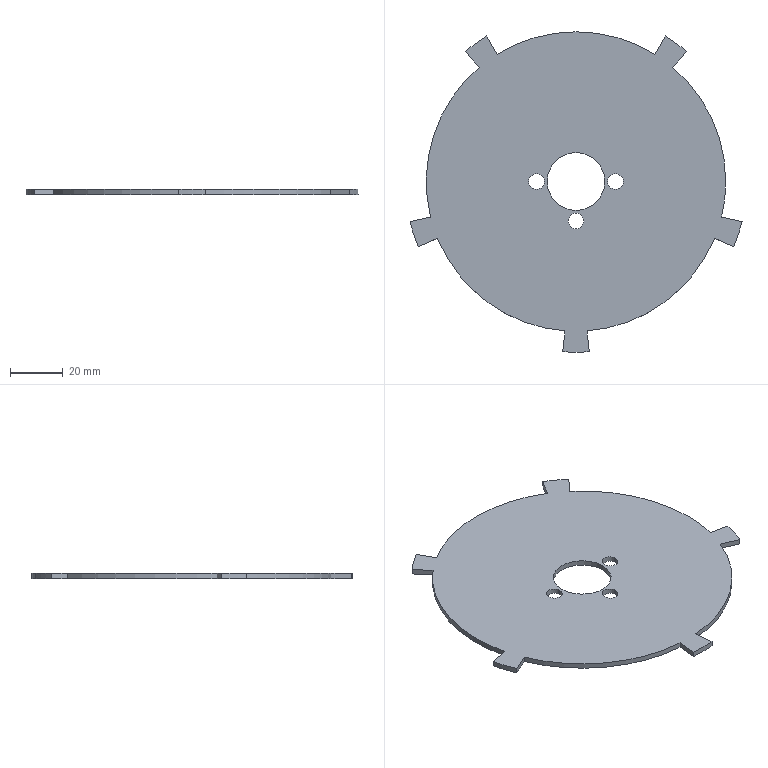Part | STEP file | 1004-2001-0084_1004-2001-0084_1-2 | 1 solid | 31 faces | box 126.387 x 122 x 2 mm | volume 20227 mm3 | cylinder 19 | plane 12 | commonest cylinder face diameters 6 x6 114 x6 130 x5 22 x2
STEP:
#1=CARTESIAN_POINT('',(-11.,0.,-1.));
#2=VERTEX_POINT('',#1);
#3=CARTESIAN_POINT('',(11.,0.,-1.));
#4=VERTEX_POINT('',#3);
#5=CARTESIAN_POINT('',(0.,0.,-1.));
#6=DIRECTION('',(0.,0.,1.));
#7=DIRECTION('',(1.,0.,0.));
#8=AXIS2_PLACEMENT_3D('',#5,#6,#7);
#9=CIRCLE('',#8,11.);
#10=EDGE_CURVE('',#2,#4,#9,.T.);
#11=ORIENTED_EDGE('',*,*,#10,.F.);
#12=CARTESIAN_POINT('',(-11.,0.,1.));
#13=VERTEX_POINT('',#12);
#14=CARTESIAN_POINT('',(-11.,0.,1.));
#15=DIRECTION('',(0.,0.,1.));
#16=VECTOR('',#15,1000.);
#17=LINE('',#14,#16);
#18=EDGE_CURVE('',#2,#13,#17,.T.);
#19=ORIENTED_EDGE('',*,*,#18,.T.);
#20=CARTESIAN_POINT('',(11.,0.,1.));
#21=VERTEX_POINT('',#20);
#22=CARTESIAN_POINT('',(0.,0.,1.));
#23=DIRECTION('',(0.,0.,-1.));
#24=DIRECTION('',(1.,0.,0.));
#25=AXIS2_PLACEMENT_3D('',#22,#23,#24);
#26=CIRCLE('',#25,11.);
#27=EDGE_CURVE('',#21,#13,#26,.T.);
#28=ORIENTED_EDGE('',*,*,#27,.F.);
#29=CARTESIAN_POINT('',(11.,0.,1.));
#30=DIRECTION('',(0.,0.,1.));
#31=VECTOR('',#30,1000.);
#32=LINE('',#29,#31);
#33=EDGE_CURVE('',#4,#21,#32,.T.);
#34=ORIENTED_EDGE('',*,*,#33,.F.);
#35=EDGE_LOOP('',(#11,#19,#28,#34));
#36=FACE_OUTER_BOUND('',#35,.T.);
#37=CARTESIAN_POINT('',(0.,0.,1.));
#38=DIRECTION('',(0.,0.,1.));
#39=DIRECTION('',(1.,0.,0.));
#40=AXIS2_PLACEMENT_3D('',#37,#38,#39);
#41=CYLINDRICAL_SURFACE('',#40,11.);
#42=ADVANCED_FACE('',(#36),#41,.F.);
#43=CARTESIAN_POINT('',(3.,-15.,1.));
#44=VERTEX_POINT('',#43);
#45=CARTESIAN_POINT('',(-3.,-15.,1.));
#46=VERTEX_POINT('',#45);
#47=CARTESIAN_POINT('',(0.,-15.,1.));
#48=DIRECTION('',(0.,0.,-1.));
#49=DIRECTION('',(-1.,0.,0.));
#50=AXIS2_PLACEMENT_3D('',#47,#48,#49);
#51=CIRCLE('',#50,3.);
#52=EDGE_CURVE('',#44,#46,#51,.T.);
#53=ORIENTED_EDGE('',*,*,#52,.F.);
#54=CARTESIAN_POINT('',(3.,-15.,-1.));
#55=VERTEX_POINT('',#54);
#56=CARTESIAN_POINT('',(3.,-15.,-1.));
#57=DIRECTION('',(0.,0.,-1.));
#58=VECTOR('',#57,1000.);
#59=LINE('',#56,#58);
#60=EDGE_CURVE('',#44,#55,#59,.T.);
#61=ORIENTED_EDGE('',*,*,#60,.T.);
#62=CARTESIAN_POINT('',(-3.,-15.,-1.));
#63=VERTEX_POINT('',#62);
#64=CARTESIAN_POINT('',(0.,-15.,-1.));
#65=DIRECTION('',(0.,0.,1.));
#66=DIRECTION('',(-1.,0.,0.));
#67=AXIS2_PLACEMENT_3D('',#64,#65,#66);
#68=CIRCLE('',#67,3.);
#69=EDGE_CURVE('',#63,#55,#68,.T.);
#70=ORIENTED_EDGE('',*,*,#69,.F.);
#71=CARTESIAN_POINT('',(-3.,-15.,-1.));
#72=DIRECTION('',(0.,0.,-1.));
#73=VECTOR('',#72,1000.);
#74=LINE('',#71,#73);
#75=EDGE_CURVE('',#46,#63,#74,.T.);
#76=ORIENTED_EDGE('',*,*,#75,.F.);
#77=EDGE_LOOP('',(#53,#61,#70,#76));
#78=FACE_OUTER_BOUND('',#77,.T.);
#79=CARTESIAN_POINT('',(0.,-15.,-1.));
#80=DIRECTION('',(0.,0.,-1.));
#81=DIRECTION('',(-1.,0.,0.));
#82=AXIS2_PLACEMENT_3D('',#79,#80,#81);
#83=CYLINDRICAL_SURFACE('',#82,3.);
#84=ADVANCED_FACE('',(#78),#83,.F.);
#85=CARTESIAN_POINT('',(-12.,0.,1.));
#86=VERTEX_POINT('',#85);
#87=CARTESIAN_POINT('',(-18.,0.,1.));
#88=VERTEX_POINT('',#87);
#89=CARTESIAN_POINT('',(-15.,0.,1.));
#90=DIRECTION('',(0.,0.,-1.));
#91=DIRECTION('',(-1.,0.,0.));
#92=AXIS2_PLACEMENT_3D('',#89,#90,#91);
#93=CIRCLE('',#92,3.);
#94=EDGE_CURVE('',#86,#88,#93,.T.);
#95=ORIENTED_EDGE('',*,*,#94,.F.);
#96=CARTESIAN_POINT('',(-12.,0.,-1.));
#97=VERTEX_POINT('',#96);
#98=CARTESIAN_POINT('',(-12.,0.,-1.));
#99=DIRECTION('',(0.,0.,-1.));
#100=VECTOR('',#99,1000.);
#101=LINE('',#98,#100);
#102=EDGE_CURVE('',#86,#97,#101,.T.);
#103=ORIENTED_EDGE('',*,*,#102,.T.);
#104=CARTESIAN_POINT('',(-18.,0.,-1.));
#105=VERTEX_POINT('',#104);
#106=CARTESIAN_POINT('',(-15.,0.,-1.));
#107=DIRECTION('',(0.,0.,1.));
#108=DIRECTION('',(-1.,0.,0.));
#109=AXIS2_PLACEMENT_3D('',#106,#107,#108);
#110=CIRCLE('',#109,3.);
#111=EDGE_CURVE('',#105,#97,#110,.T.);
#112=ORIENTED_EDGE('',*,*,#111,.F.);
#113=CARTESIAN_POINT('',(-18.,0.,-1.));
#114=DIRECTION('',(0.,0.,-1.));
#115=VECTOR('',#114,1000.);
#116=LINE('',#113,#115);
#117=EDGE_CURVE('',#88,#105,#116,.T.);
#118=ORIENTED_EDGE('',*,*,#117,.F.);
#119=EDGE_LOOP('',(#95,#103,#112,#118));
#120=FACE_OUTER_BOUND('',#119,.T.);
#121=CARTESIAN_POINT('',(-15.,0.,-1.));
#122=DIRECTION('',(0.,0.,-1.));
#123=DIRECTION('',(-1.,0.,0.));
#124=AXIS2_PLACEMENT_3D('',#121,#122,#123);
#125=CYLINDRICAL_SURFACE('',#124,3.);
#126=ADVANCED_FACE('',(#120),#125,.F.);
#127=CARTESIAN_POINT('',(18.,0.,1.));
#128=VERTEX_POINT('',#127);
#129=CARTESIAN_POINT('',(12.,0.,1.));
#130=VERTEX_POINT('',#129);
#131=CARTESIAN_POINT('',(15.,0.,1.));
#132=DIRECTION('',(0.,0.,-1.));
#133=DIRECTION('',(-1.,0.,0.));
#134=AXIS2_PLACEMENT_3D('',#131,#132,#133);
#135=CIRCLE('',#134,3.);
#136=EDGE_CURVE('',#128,#130,#135,.T.);
#137=ORIENTED_EDGE('',*,*,#136,.F.);
#138=CARTESIAN_POINT('',(18.,0.,-1.));
#139=VERTEX_POINT('',#138);
#140=CARTESIAN_POINT('',(18.,0.,-1.));
#141=DIRECTION('',(0.,0.,-1.));
#142=VECTOR('',#141,1000.);
#143=LINE('',#140,#142);
#144=EDGE_CURVE('',#128,#139,#143,.T.);
#145=ORIENTED_EDGE('',*,*,#144,.T.);
#146=CARTESIAN_POINT('',(12.,0.,-1.));
#147=VERTEX_POINT('',#146);
#148=CARTESIAN_POINT('',(15.,0.,-1.));
#149=DIRECTION('',(0.,0.,1.));
#150=DIRECTION('',(-1.,0.,0.));
#151=AXIS2_PLACEMENT_3D('',#148,#149,#150);
#152=CIRCLE('',#151,3.);
#153=EDGE_CURVE('',#147,#139,#152,.T.);
#154=ORIENTED_EDGE('',*,*,#153,.F.);
#155=CARTESIAN_POINT('',(12.,0.,-1.));
#156=DIRECTION('',(0.,0.,-1.));
#157=VECTOR('',#156,1000.);
#158=LINE('',#155,#157);
#159=EDGE_CURVE('',#130,#147,#158,.T.);
#160=ORIENTED_EDGE('',*,*,#159,.F.);
#161=EDGE_LOOP('',(#137,#145,#154,#160));
#162=FACE_OUTER_BOUND('',#161,.T.);
#163=CARTESIAN_POINT('',(15.,0.,-1.));
#164=DIRECTION('',(0.,0.,-1.));
#165=DIRECTION('',(-1.,0.,0.));
#166=AXIS2_PLACEMENT_3D('',#163,#164,#165);
#167=CYLINDRICAL_SURFACE('',#166,3.);
#168=ADVANCED_FACE('',(#162),#167,.F.);
#169=CARTESIAN_POINT('',(55.365,-13.555,-1.));
#170=VERTEX_POINT('',#169);
#171=CARTESIAN_POINT('',(57.,0.,-1.));
#172=VERTEX_POINT('',#171);
#173=CARTESIAN_POINT('',(0.,0.,-1.));
#174=DIRECTION('',(0.,0.,1.));
#175=DIRECTION('',(1.,0.,0.));
#176=AXIS2_PLACEMENT_3D('',#173,#174,#175);
#177=CIRCLE('',#176,57.);
#178=EDGE_CURVE('',#170,#172,#177,.T.);
#179=ORIENTED_EDGE('',*,*,#178,.T.);
#180=CARTESIAN_POINT('',(57.,0.,1.));
#181=VERTEX_POINT('',#180);
#182=CARTESIAN_POINT('',(57.,0.,-1.));
#183=DIRECTION('',(0.,0.,1.));
#184=VECTOR('',#183,1000.);
#185=LINE('',#182,#184);
#186=EDGE_CURVE('',#172,#181,#185,.T.);
#187=ORIENTED_EDGE('',*,*,#186,.T.);
#188=CARTESIAN_POINT('',(55.365,-13.555,1.));
#189=VERTEX_POINT('',#188);
#190=CARTESIAN_POINT('',(0.,0.,1.));
#191=DIRECTION('',(0.,0.,1.));
#192=DIRECTION('',(1.,0.,0.));
#193=AXIS2_PLACEMENT_3D('',#190,#191,#192);
#194=CIRCLE('',#193,57.);
#195=EDGE_CURVE('',#189,#181,#194,.T.);
#196=ORIENTED_EDGE('',*,*,#195,.F.);
#197=CARTESIAN_POINT('',(55.365,-13.555,-1.));
#198=DIRECTION('',(0.,0.,-1.));
#199=VECTOR('',#198,1000.);
#200=LINE('',#197,#199);
#201=EDGE_CURVE('',#189,#170,#200,.T.);
#202=ORIENTED_EDGE('',*,*,#201,.T.);
#203=EDGE_LOOP('',(#179,#187,#196,#202));
#204=FACE_OUTER_BOUND('',#203,.T.);
#205=CARTESIAN_POINT('',(0.,0.,-1.));
#206=DIRECTION('',(0.,0.,1.));
#207=DIRECTION('',(1.,0.,0.));
#208=AXIS2_PLACEMENT_3D('',#205,#206,#207);
#209=CYLINDRICAL_SURFACE('',#208,57.);
#210=ADVANCED_FACE('',(#204),#209,.T.);
#211=ORIENTED_EDGE('',*,*,#27,.T.);
#212=CARTESIAN_POINT('',(0.,0.,1.));
#213=DIRECTION('',(0.,0.,-1.));
#214=DIRECTION('',(1.,0.,0.));
#215=AXIS2_PLACEMENT_3D('',#212,#213,#214);
#216=CIRCLE('',#215,11.);
#217=EDGE_CURVE('',#13,#21,#216,.T.);
#218=ORIENTED_EDGE('',*,*,#217,.T.);
#219=EDGE_LOOP('',(#211,#218));
#220=FACE_BOUND('',#219,.T.);
#221=CARTESIAN_POINT('',(0.,-15.,1.));
#222=DIRECTION('',(0.,0.,-1.));
#223=DIRECTION('',(-1.,0.,0.));
#224=AXIS2_PLACEMENT_3D('',#221,#222,#223);
#225=CIRCLE('',#224,3.);
#226=EDGE_CURVE('',#46,#44,#225,.T.);
#227=ORIENTED_EDGE('',*,*,#226,.T.);
#228=ORIENTED_EDGE('',*,*,#52,.T.);
#229=EDGE_LOOP('',(#227,#228));
#230=FACE_BOUND('',#229,.T.);
#231=CARTESIAN_POINT('',(-15.,0.,1.));
#232=DIRECTION('',(0.,0.,-1.));
#233=DIRECTION('',(-1.,0.,0.));
#234=AXIS2_PLACEMENT_3D('',#231,#232,#233);
#235=CIRCLE('',#234,3.);
#236=EDGE_CURVE('',#88,#86,#235,.T.);
#237=ORIENTED_EDGE('',*,*,#236,.T.);
#238=ORIENTED_EDGE('',*,*,#94,.T.);
#239=EDGE_LOOP('',(#237,#238));
#240=FACE_BOUND('',#239,.T.);
#241=CARTESIAN_POINT('',(15.,0.,1.));
#242=DIRECTION('',(0.,0.,-1.));
#243=DIRECTION('',(-1.,0.,0.));
#244=AXIS2_PLACEMENT_3D('',#241,#242,#243);
#245=CIRCLE('',#244,3.);
#246=EDGE_CURVE('',#130,#128,#245,.T.);
#247=ORIENTED_EDGE('',*,*,#246,.T.);
#248=ORIENTED_EDGE('',*,*,#136,.T.);
#249=EDGE_LOOP('',(#247,#248));
#250=FACE_BOUND('',#249,.T.);
#251=CARTESIAN_POINT('',(-36.824,43.509,1.));
#252=VERTEX_POINT('',#251);
#253=CARTESIAN_POINT('',(-55.365,-13.555,1.));
#254=VERTEX_POINT('',#253);
#255=CARTESIAN_POINT('',(0.,0.,1.));
#256=DIRECTION('',(0.,0.,1.));
#257=DIRECTION('',(1.,0.,0.));
#258=AXIS2_PLACEMENT_3D('',#255,#256,#257);
#259=CIRCLE('',#258,57.);
#260=EDGE_CURVE('',#252,#254,#259,.T.);
#261=ORIENTED_EDGE('',*,*,#260,.T.);
#262=CARTESIAN_POINT('',(-63.193,-15.219,1.));
#263=VERTEX_POINT('',#262);
#264=CARTESIAN_POINT('',(-55.365,-13.555,1.));
#265=DIRECTION('',(-0.9781,-0.2079,0.));
#266=VECTOR('',#265,1000.);
#267=LINE('',#264,#266);
#268=EDGE_CURVE('',#254,#263,#267,.T.);
#269=ORIENTED_EDGE('',*,*,#268,.T.);
#270=CARTESIAN_POINT('',(-60.07,-24.832,1.));
#271=VERTEX_POINT('',#270);
#272=CARTESIAN_POINT('',(0.,0.,1.));
#273=DIRECTION('',(0.,0.,1.));
#274=DIRECTION('',(-1.,0.,0.));
#275=AXIS2_PLACEMENT_3D('',#272,#273,#274);
#276=CIRCLE('',#275,65.);
#277=EDGE_CURVE('',#263,#271,#276,.T.);
#278=ORIENTED_EDGE('',*,*,#277,.T.);
#279=CARTESIAN_POINT('',(-52.758,-21.577,1.));
#280=VERTEX_POINT('',#279);
#281=CARTESIAN_POINT('',(-60.07,-24.832,1.));
#282=DIRECTION('',(0.9135,0.4067,0.));
#283=VECTOR('',#282,1000.);
#284=LINE('',#281,#283);
#285=EDGE_CURVE('',#271,#280,#284,.T.);
#286=ORIENTED_EDGE('',*,*,#285,.T.);
#287=CARTESIAN_POINT('',(-4.217,-56.844,1.));
#288=VERTEX_POINT('',#287);
#289=CARTESIAN_POINT('',(0.,0.,1.));
#290=DIRECTION('',(0.,0.,1.));
#291=DIRECTION('',(1.,0.,0.));
#292=AXIS2_PLACEMENT_3D('',#289,#290,#291);
#293=CIRCLE('',#292,57.);
#294=EDGE_CURVE('',#280,#288,#293,.T.);
#295=ORIENTED_EDGE('',*,*,#294,.T.);
#296=CARTESIAN_POINT('',(-5.054,-64.803,1.));
#297=VERTEX_POINT('',#296);
#298=CARTESIAN_POINT('',(-4.217,-56.844,1.));
#299=DIRECTION('',(-0.1045,-0.9945,0.));
#300=VECTOR('',#299,1000.);
#301=LINE('',#298,#300);
#302=EDGE_CURVE('',#288,#297,#301,.T.);
#303=ORIENTED_EDGE('',*,*,#302,.T.);
#304=CARTESIAN_POINT('',(5.054,-64.803,1.));
#305=VERTEX_POINT('',#304);
#306=CARTESIAN_POINT('',(0.,0.,1.));
#307=DIRECTION('',(0.,0.,1.));
#308=DIRECTION('',(-1.,0.,0.));
#309=AXIS2_PLACEMENT_3D('',#306,#307,#308);
#310=CIRCLE('',#309,65.);
#311=EDGE_CURVE('',#297,#305,#310,.T.);
#312=ORIENTED_EDGE('',*,*,#311,.T.);
#313=CARTESIAN_POINT('',(4.217,-56.844,1.));
#314=VERTEX_POINT('',#313);
#315=CARTESIAN_POINT('',(5.054,-64.803,1.));
#316=DIRECTION('',(-0.1045,0.9945,0.));
#317=VECTOR('',#316,1000.);
#318=LINE('',#315,#317);
#319=EDGE_CURVE('',#305,#314,#318,.T.);
#320=ORIENTED_EDGE('',*,*,#319,.T.);
#321=CARTESIAN_POINT('',(52.758,-21.577,1.));
#322=VERTEX_POINT('',#321);
#323=CARTESIAN_POINT('',(0.,0.,1.));
#324=DIRECTION('',(0.,0.,1.));
#325=DIRECTION('',(1.,0.,0.));
#326=AXIS2_PLACEMENT_3D('',#323,#324,#325);
#327=CIRCLE('',#326,57.);
#328=EDGE_CURVE('',#314,#322,#327,.T.);
#329=ORIENTED_EDGE('',*,*,#328,.T.);
#330=CARTESIAN_POINT('',(60.07,-24.832,1.));
#331=VERTEX_POINT('',#330);
#332=CARTESIAN_POINT('',(52.758,-21.577,1.));
#333=DIRECTION('',(0.9135,-0.4067,0.));
#334=VECTOR('',#333,1000.);
#335=LINE('',#332,#334);
#336=EDGE_CURVE('',#322,#331,#335,.T.);
#337=ORIENTED_EDGE('',*,*,#336,.T.);
#338=CARTESIAN_POINT('',(63.193,-15.219,1.));
#339=VERTEX_POINT('',#338);
#340=CARTESIAN_POINT('',(0.,0.,1.));
#341=DIRECTION('',(0.,0.,1.));
#342=DIRECTION('',(-1.,0.,0.));
#343=AXIS2_PLACEMENT_3D('',#340,#341,#342);
#344=CIRCLE('',#343,65.);
#345=EDGE_CURVE('',#331,#339,#344,.T.);
#346=ORIENTED_EDGE('',*,*,#345,.T.);
#347=CARTESIAN_POINT('',(63.193,-15.219,1.));
#348=DIRECTION('',(-0.9781,0.2079,0.));
#349=VECTOR('',#348,1000.);
#350=LINE('',#347,#349);
#351=EDGE_CURVE('',#339,#189,#350,.T.);
#352=ORIENTED_EDGE('',*,*,#351,.T.);
#353=ORIENTED_EDGE('',*,*,#195,.T.);
#354=CARTESIAN_POINT('',(36.824,43.509,1.));
#355=VERTEX_POINT('',#354);
#356=CARTESIAN_POINT('',(0.,0.,1.));
#357=DIRECTION('',(0.,0.,1.));
#358=DIRECTION('',(1.,0.,0.));
#359=AXIS2_PLACEMENT_3D('',#356,#357,#358);
#360=CIRCLE('',#359,57.);
#361=EDGE_CURVE('',#181,#355,#360,.T.);
#362=ORIENTED_EDGE('',*,*,#361,.T.);
#363=CARTESIAN_POINT('',(42.179,49.456,1.));
#364=VERTEX_POINT('',#363);
#365=CARTESIAN_POINT('',(36.824,43.509,1.));
#366=DIRECTION('',(0.6691,0.7431,0.));
#367=VECTOR('',#366,1000.);
#368=LINE('',#365,#367);
#369=EDGE_CURVE('',#355,#364,#368,.T.);
#370=ORIENTED_EDGE('',*,*,#369,.T.);
#371=CARTESIAN_POINT('',(34.002,55.398,1.));
#372=VERTEX_POINT('',#371);
#373=CARTESIAN_POINT('',(0.,0.,1.));
#374=DIRECTION('',(0.,0.,1.));
#375=DIRECTION('',(-1.,0.,0.));
#376=AXIS2_PLACEMENT_3D('',#373,#374,#375);
#377=CIRCLE('',#376,65.);
#378=EDGE_CURVE('',#364,#372,#377,.T.);
#379=ORIENTED_EDGE('',*,*,#378,.T.);
#380=CARTESIAN_POINT('',(30.,48.466,1.));
#381=VERTEX_POINT('',#380);
#382=CARTESIAN_POINT('',(34.002,55.398,1.));
#383=DIRECTION('',(-0.5,-0.866,0.));
#384=VECTOR('',#383,1000.);
#385=LINE('',#382,#384);
#386=EDGE_CURVE('',#372,#381,#385,.T.);
#387=ORIENTED_EDGE('',*,*,#386,.T.);
#388=CARTESIAN_POINT('',(-30.,48.466,1.));
#389=VERTEX_POINT('',#388);
#390=CARTESIAN_POINT('',(0.,0.,1.));
#391=DIRECTION('',(0.,0.,1.));
#392=DIRECTION('',(1.,0.,0.));
#393=AXIS2_PLACEMENT_3D('',#390,#391,#392);
#394=CIRCLE('',#393,57.);
#395=EDGE_CURVE('',#381,#389,#394,.T.);
#396=ORIENTED_EDGE('',*,*,#395,.T.);
#397=CARTESIAN_POINT('',(-34.002,55.398,1.));
#398=VERTEX_POINT('',#397);
#399=CARTESIAN_POINT('',(-30.,48.466,1.));
#400=DIRECTION('',(-0.5,0.866,0.));
#401=VECTOR('',#400,1000.);
#402=LINE('',#399,#401);
#403=EDGE_CURVE('',#389,#398,#402,.T.);
#404=ORIENTED_EDGE('',*,*,#403,.T.);
#405=CARTESIAN_POINT('',(-42.179,49.456,1.));
#406=VERTEX_POINT('',#405);
#407=CARTESIAN_POINT('',(0.,0.,1.));
#408=DIRECTION('',(0.,0.,1.));
#409=DIRECTION('',(-1.,0.,0.));
#410=AXIS2_PLACEMENT_3D('',#407,#408,#409);
#411=CIRCLE('',#410,65.);
#412=EDGE_CURVE('',#398,#406,#411,.T.);
#413=ORIENTED_EDGE('',*,*,#412,.T.);
#414=CARTESIAN_POINT('',(-42.179,49.456,1.));
#415=DIRECTION('',(0.6691,-0.7431,0.));
#416=VECTOR('',#415,1000.);
#417=LINE('',#414,#416);
#418=EDGE_CURVE('',#406,#252,#417,.T.);
#419=ORIENTED_EDGE('',*,*,#418,.T.);
#420=EDGE_LOOP('',(#261,#269,#278,#286,#295,#303,#312,#320,#329,#337,#346,#352,#353,#362,#370,#379,#387,#396,#404,#413,#419));
#421=FACE_OUTER_BOUND('',#420,.T.);
#422=CARTESIAN_POINT('',(0.,0.,1.));
#423=DIRECTION('',(0.,0.,1.));
#424=DIRECTION('',(1.,0.,0.));
#425=AXIS2_PLACEMENT_3D('',#422,#423,#424);
#426=PLANE('',#425);
#427=ADVANCED_FACE('',(#220,#230,#240,#250,#421),#426,.T.);
#428=ORIENTED_EDGE('',*,*,#18,.F.);
#429=CARTESIAN_POINT('',(0.,0.,-1.));
#430=DIRECTION('',(0.,0.,1.));
#431=DIRECTION('',(1.,0.,0.));
#432=AXIS2_PLACEMENT_3D('',#429,#430,#431);
#433=CIRCLE('',#432,11.);
#434=EDGE_CURVE('',#4,#2,#433,.T.);
#435=ORIENTED_EDGE('',*,*,#434,.F.);
#436=ORIENTED_EDGE('',*,*,#33,.T.);
#437=ORIENTED_EDGE('',*,*,#217,.F.);
#438=EDGE_LOOP('',(#428,#435,#436,#437));
#439=FACE_OUTER_BOUND('',#438,.T.);
#440=CARTESIAN_POINT('',(0.,0.,1.));
#441=DIRECTION('',(0.,0.,1.));
#442=DIRECTION('',(1.,0.,0.));
#443=AXIS2_PLACEMENT_3D('',#440,#441,#442);
#444=CYLINDRICAL_SURFACE('',#443,11.);
#445=ADVANCED_FACE('',(#439),#444,.F.);
#446=ORIENTED_EDGE('',*,*,#60,.F.);
#447=ORIENTED_EDGE('',*,*,#226,.F.);
#448=ORIENTED_EDGE('',*,*,#75,.T.);
#449=CARTESIAN_POINT('',(0.,-15.,-1.));
#450=DIRECTION('',(0.,0.,1.));
#451=DIRECTION('',(-1.,0.,0.));
#452=AXIS2_PLACEMENT_3D('',#449,#450,#451);
#453=CIRCLE('',#452,3.);
#454=EDGE_CURVE('',#55,#63,#453,.T.);
#455=ORIENTED_EDGE('',*,*,#454,.F.);
#456=EDGE_LOOP('',(#446,#447,#448,#455));
#457=FACE_OUTER_BOUND('',#456,.T.);
#458=CARTESIAN_POINT('',(0.,-15.,-1.));
#459=DIRECTION('',(0.,0.,-1.));
#460=DIRECTION('',(-1.,0.,0.));
#461=AXIS2_PLACEMENT_3D('',#458,#459,#460);
#462=CYLINDRICAL_SURFACE('',#461,3.);
#463=ADVANCED_FACE('',(#457),#462,.F.);
#464=ORIENTED_EDGE('',*,*,#102,.F.);
#465=ORIENTED_EDGE('',*,*,#236,.F.);
#466=ORIENTED_EDGE('',*,*,#117,.T.);
#467=CARTESIAN_POINT('',(-15.,0.,-1.));
#468=DIRECTION('',(0.,0.,1.));
#469=DIRECTION('',(-1.,0.,0.));
#470=AXIS2_PLACEMENT_3D('',#467,#468,#469);
#471=CIRCLE('',#470,3.);
#472=EDGE_CURVE('',#97,#105,#471,.T.);
#473=ORIENTED_EDGE('',*,*,#472,.F.);
#474=EDGE_LOOP('',(#464,#465,#466,#473));
#475=FACE_OUTER_BOUND('',#474,.T.);
#476=CARTESIAN_POINT('',(-15.,0.,-1.));
#477=DIRECTION('',(0.,0.,-1.));
#478=DIRECTION('',(-1.,0.,0.));
#479=AXIS2_PLACEMENT_3D('',#476,#477,#478);
#480=CYLINDRICAL_SURFACE('',#479,3.);
#481=ADVANCED_FACE('',(#475),#480,.F.);
#482=ORIENTED_EDGE('',*,*,#144,.F.);
#483=ORIENTED_EDGE('',*,*,#246,.F.);
#484=ORIENTED_EDGE('',*,*,#159,.T.);
#485=CARTESIAN_POINT('',(15.,0.,-1.));
#486=DIRECTION('',(0.,0.,1.));
#487=DIRECTION('',(-1.,0.,0.));
#488=AXIS2_PLACEMENT_3D('',#485,#486,#487);
#489=CIRCLE('',#488,3.);
#490=EDGE_CURVE('',#139,#147,#489,.T.);
#491=ORIENTED_EDGE('',*,*,#490,.F.);
#492=EDGE_LOOP('',(#482,#483,#484,#491));
#493=FACE_OUTER_BOUND('',#492,.T.);
#494=CARTESIAN_POINT('',(15.,0.,-1.));
#495=DIRECTION('',(0.,0.,-1.));
#496=DIRECTION('',(-1.,0.,0.));
#497=AXIS2_PLACEMENT_3D('',#494,#495,#496);
#498=CYLINDRICAL_SURFACE('',#497,3.);
#499=ADVANCED_FACE('',(#493),#498,.F.);
#500=CARTESIAN_POINT('',(-63.193,-15.219,-1.));
#501=VERTEX_POINT('',#500);
#502=CARTESIAN_POINT('',(-55.365,-13.555,-1.));
#503=VERTEX_POINT('',#502);
#504=CARTESIAN_POINT('',(-55.365,-13.555,-1.));
#505=DIRECTION('',(0.9781,0.2079,0.));
#506=VECTOR('',#505,1000.);
#507=LINE('',#504,#506);
#508=EDGE_CURVE('',#501,#503,#507,.T.);
#509=ORIENTED_EDGE('',*,*,#508,.F.);
#510=CARTESIAN_POINT('',(-63.193,-15.219,-1.));
#511=DIRECTION('',(0.,0.,-1.));
#512=VECTOR('',#511,1000.);
#513=LINE('',#510,#512);
#514=EDGE_CURVE('',#263,#501,#513,.T.);
#515=ORIENTED_EDGE('',*,*,#514,.F.);
#516=ORIENTED_EDGE('',*,*,#268,.F.);
#517=CARTESIAN_POINT('',(-55.365,-13.555,-1.));
#518=DIRECTION('',(0.,0.,1.));
#519=VECTOR('',#518,1000.);
#520=LINE('',#517,#519);
#521=EDGE_CURVE('',#503,#254,#520,.T.);
#522=ORIENTED_EDGE('',*,*,#521,.F.);
#523=EDGE_LOOP('',(#509,#515,#516,#522));
#524=FACE_OUTER_BOUND('',#523,.T.);
#525=CARTESIAN_POINT('',(-55.365,-13.555,-1.));
#526=DIRECTION('',(0.2079,-0.9781,0.));
#527=DIRECTION('',(0.9781,0.2079,0.));
#528=AXIS2_PLACEMENT_3D('',#525,#526,#527);
#529=PLANE('',#528);
#530=ADVANCED_FACE('',(#524),#529,.F.);
#531=ORIENTED_EDGE('',*,*,#521,.T.);
#532=ORIENTED_EDGE('',*,*,#260,.F.);
#533=CARTESIAN_POINT('',(-36.824,43.509,-1.));
#534=VERTEX_POINT('',#533);
#535=CARTESIAN_POINT('',(-36.824,43.509,-1.));
#536=DIRECTION('',(0.,0.,-1.));
#537=VECTOR('',#536,1000.);
#538=LINE('',#535,#537);
#539=EDGE_CURVE('',#252,#534,#538,.T.);
#540=ORIENTED_EDGE('',*,*,#539,.T.);
#541=CARTESIAN_POINT('',(0.,0.,-1.));
#542=DIRECTION('',(0.,0.,1.));
#543=DIRECTION('',(1.,0.,0.));
#544=AXIS2_PLACEMENT_3D('',#541,#542,#543);
#545=CIRCLE('',#544,57.);
#546=EDGE_CURVE('',#534,#503,#545,.T.);
#547=ORIENTED_EDGE('',*,*,#546,.T.);
#548=EDGE_LOOP('',(#531,#532,#540,#547));
#549=FACE_OUTER_BOUND('',#548,.T.);
#550=CARTESIAN_POINT('',(0.,0.,-1.));
#551=DIRECTION('',(0.,0.,1.));
#552=DIRECTION('',(1.,0.,0.));
#553=AXIS2_PLACEMENT_3D('',#550,#551,#552);
#554=CYLINDRICAL_SURFACE('',#553,57.);
#555=ADVANCED_FACE('',(#549),#554,.T.);
#556=CARTESIAN_POINT('',(-42.179,49.456,-1.));
#557=VERTEX_POINT('',#556);
#558=CARTESIAN_POINT('',(-36.824,43.509,-1.));
#559=DIRECTION('',(-0.6691,0.7431,0.));
#560=VECTOR('',#559,1000.);
#561=LINE('',#558,#560);
#562=EDGE_CURVE('',#534,#557,#561,.T.);
#563=ORIENTED_EDGE('',*,*,#562,.F.);
#564=ORIENTED_EDGE('',*,*,#539,.F.);
#565=ORIENTED_EDGE('',*,*,#418,.F.);
#566=CARTESIAN_POINT('',(-42.179,49.456,-1.));
#567=DIRECTION('',(0.,0.,1.));
#568=VECTOR('',#567,1000.);
#569=LINE('',#566,#568);
#570=EDGE_CURVE('',#557,#406,#569,.T.);
#571=ORIENTED_EDGE('',*,*,#570,.F.);
#572=EDGE_LOOP('',(#563,#564,#565,#571));
#573=FACE_OUTER_BOUND('',#572,.T.);
#574=CARTESIAN_POINT('',(-36.824,43.509,-1.));
#575=DIRECTION('',(0.7431,0.6691,0.));
#576=DIRECTION('',(-0.6691,0.7431,0.));
#577=AXIS2_PLACEMENT_3D('',#574,#575,#576);
#578=PLANE('',#577);
#579=ADVANCED_FACE('',(#573),#578,.F.);
#580=CARTESIAN_POINT('',(-34.002,55.398,-1.));
#581=VERTEX_POINT('',#580);
#582=CARTESIAN_POINT('',(-34.002,55.398,1.));
#583=DIRECTION('',(0.,0.,-1.));
#584=VECTOR('',#583,1000.);
#585=LINE('',#582,#584);
#586=EDGE_CURVE('',#398,#581,#585,.T.);
#587=ORIENTED_EDGE('',*,*,#586,.T.);
#588=CARTESIAN_POINT('',(0.,0.,-1.));
#589=DIRECTION('',(0.,0.,1.));
#590=DIRECTION('',(-1.,0.,0.));
#591=AXIS2_PLACEMENT_3D('',#588,#589,#590);
#592=CIRCLE('',#591,65.);
#593=EDGE_CURVE('',#581,#557,#592,.T.);
#594=ORIENTED_EDGE('',*,*,#593,.T.);
#595=ORIENTED_EDGE('',*,*,#570,.T.);
#596=ORIENTED_EDGE('',*,*,#412,.F.);
#597=EDGE_LOOP('',(#587,#594,#595,#596));
#598=FACE_OUTER_BOUND('',#597,.T.);
#599=CARTESIAN_POINT('',(0.,0.,1.));
#600=DIRECTION('',(0.,0.,-1.));
#601=DIRECTION('',(-1.,0.,0.));
#602=AXIS2_PLACEMENT_3D('',#599,#600,#601);
#603=CYLINDRICAL_SURFACE('',#602,65.);
#604=ADVANCED_FACE('',(#598),#603,.T.);
#605=CARTESIAN_POINT('',(-30.,48.466,-1.));
#606=VERTEX_POINT('',#605);
#607=CARTESIAN_POINT('',(-30.,48.466,-1.));
#608=DIRECTION('',(0.5,-0.866,0.));
#609=VECTOR('',#608,1000.);
#610=LINE('',#607,#609);
#611=EDGE_CURVE('',#581,#606,#610,.T.);
#612=ORIENTED_EDGE('',*,*,#611,.F.);
#613=ORIENTED_EDGE('',*,*,#586,.F.);
#614=ORIENTED_EDGE('',*,*,#403,.F.);
#615=CARTESIAN_POINT('',(-30.,48.466,-1.));
#616=DIRECTION('',(0.,0.,1.));
#617=VECTOR('',#616,1000.);
#618=LINE('',#615,#617);
#619=EDGE_CURVE('',#606,#389,#618,.T.);
#620=ORIENTED_EDGE('',*,*,#619,.F.);
#621=EDGE_LOOP('',(#612,#613,#614,#620));
#622=FACE_OUTER_BOUND('',#621,.T.);
#623=CARTESIAN_POINT('',(-30.,48.466,-1.));
#624=DIRECTION('',(-0.866,-0.5,0.));
#625=DIRECTION('',(0.5,-0.866,0.));
#626=AXIS2_PLACEMENT_3D('',#623,#624,#625);
#627=PLANE('',#626);
#628=ADVANCED_FACE('',(#622),#627,.F.);
#629=ORIENTED_EDGE('',*,*,#619,.T.);
#630=ORIENTED_EDGE('',*,*,#395,.F.);
#631=CARTESIAN_POINT('',(30.,48.466,-1.));
#632=VERTEX_POINT('',#631);
#633=CARTESIAN_POINT('',(30.,48.466,-1.));
#634=DIRECTION('',(0.,0.,-1.));
#635=VECTOR('',#634,1000.);
#636=LINE('',#633,#635);
#637=EDGE_CURVE('',#381,#632,#636,.T.);
#638=ORIENTED_EDGE('',*,*,#637,.T.);
#639=CARTESIAN_POINT('',(0.,0.,-1.));
#640=DIRECTION('',(0.,0.,1.));
#641=DIRECTION('',(1.,0.,0.));
#642=AXIS2_PLACEMENT_3D('',#639,#640,#641);
#643=CIRCLE('',#642,57.);
#644=EDGE_CURVE('',#632,#606,#643,.T.);
#645=ORIENTED_EDGE('',*,*,#644,.T.);
#646=EDGE_LOOP('',(#629,#630,#638,#645));
#647=FACE_OUTER_BOUND('',#646,.T.);
#648=CARTESIAN_POINT('',(0.,0.,-1.));
#649=DIRECTION('',(0.,0.,1.));
#650=DIRECTION('',(1.,0.,0.));
#651=AXIS2_PLACEMENT_3D('',#648,#649,#650);
#652=CYLINDRICAL_SURFACE('',#651,57.);
#653=ADVANCED_FACE('',(#647),#652,.T.);
#654=CARTESIAN_POINT('',(34.002,55.398,-1.));
#655=VERTEX_POINT('',#654);
#656=CARTESIAN_POINT('',(30.,48.466,-1.));
#657=DIRECTION('',(0.5,0.866,0.));
#658=VECTOR('',#657,1000.);
#659=LINE('',#656,#658);
#660=EDGE_CURVE('',#632,#655,#659,.T.);
#661=ORIENTED_EDGE('',*,*,#660,.F.);
#662=ORIENTED_EDGE('',*,*,#637,.F.);
#663=ORIENTED_EDGE('',*,*,#386,.F.);
#664=CARTESIAN_POINT('',(34.002,55.398,-1.));
#665=DIRECTION('',(0.,0.,1.));
#666=VECTOR('',#665,1000.);
#667=LINE('',#664,#666);
#668=EDGE_CURVE('',#655,#372,#667,.T.);
#669=ORIENTED_EDGE('',*,*,#668,.F.);
#670=EDGE_LOOP('',(#661,#662,#663,#669));
#671=FACE_OUTER_BOUND('',#670,.T.);
#672=CARTESIAN_POINT('',(30.,48.466,-1.));
#673=DIRECTION('',(0.866,-0.5,0.));
#674=DIRECTION('',(0.5,0.866,0.));
#675=AXIS2_PLACEMENT_3D('',#672,#673,#674);
#676=PLANE('',#675);
#677=ADVANCED_FACE('',(#671),#676,.F.);
#678=ORIENTED_EDGE('',*,*,#668,.T.);
#679=ORIENTED_EDGE('',*,*,#378,.F.);
#680=CARTESIAN_POINT('',(42.179,49.456,-1.));
#681=VERTEX_POINT('',#680);
#682=CARTESIAN_POINT('',(42.179,49.456,1.));
#683=DIRECTION('',(0.,0.,-1.));
#684=VECTOR('',#683,1000.);
#685=LINE('',#682,#684);
#686=EDGE_CURVE('',#364,#681,#685,.T.);
#687=ORIENTED_EDGE('',*,*,#686,.T.);
#688=CARTESIAN_POINT('',(0.,0.,-1.));
#689=DIRECTION('',(0.,0.,1.));
#690=DIRECTION('',(-1.,0.,0.));
#691=AXIS2_PLACEMENT_3D('',#688,#689,#690);
#692=CIRCLE('',#691,65.);
#693=EDGE_CURVE('',#681,#655,#692,.T.);
#694=ORIENTED_EDGE('',*,*,#693,.T.);
#695=EDGE_LOOP('',(#678,#679,#687,#694));
#696=FACE_OUTER_BOUND('',#695,.T.);
#697=CARTESIAN_POINT('',(0.,0.,1.));
#698=DIRECTION('',(0.,0.,-1.));
#699=DIRECTION('',(-1.,0.,0.));
#700=AXIS2_PLACEMENT_3D('',#697,#698,#699);
#701=CYLINDRICAL_SURFACE('',#700,65.);
#702=ADVANCED_FACE('',(#696),#701,.T.);
#703=CARTESIAN_POINT('',(36.824,43.509,-1.));
#704=VERTEX_POINT('',#703);
#705=CARTESIAN_POINT('',(36.824,43.509,-1.));
#706=DIRECTION('',(-0.6691,-0.7431,0.));
#707=VECTOR('',#706,1000.);
#708=LINE('',#705,#707);
#709=EDGE_CURVE('',#681,#704,#708,.T.);
#710=ORIENTED_EDGE('',*,*,#709,.F.);
#711=ORIENTED_EDGE('',*,*,#686,.F.);
#712=ORIENTED_EDGE('',*,*,#369,.F.);
#713=CARTESIAN_POINT('',(36.824,43.509,-1.));
#714=DIRECTION('',(0.,0.,1.));
#715=VECTOR('',#714,1000.);
#716=LINE('',#713,#715);
#717=EDGE_CURVE('',#704,#355,#716,.T.);
#718=ORIENTED_EDGE('',*,*,#717,.F.);
#719=EDGE_LOOP('',(#710,#711,#712,#718));
#720=FACE_OUTER_BOUND('',#719,.T.);
#721=CARTESIAN_POINT('',(36.824,43.509,-1.));
#722=DIRECTION('',(-0.7431,0.6691,0.));
#723=DIRECTION('',(-0.6691,-0.7431,0.));
#724=AXIS2_PLACEMENT_3D('',#721,#722,#723);
#725=PLANE('',#724);
#726=ADVANCED_FACE('',(#720),#725,.F.);
#727=ORIENTED_EDGE('',*,*,#186,.F.);
#728=CARTESIAN_POINT('',(0.,0.,-1.));
#729=DIRECTION('',(0.,0.,1.));
#730=DIRECTION('',(1.,0.,0.));
#731=AXIS2_PLACEMENT_3D('',#728,#729,#730);
#732=CIRCLE('',#731,57.);
#733=EDGE_CURVE('',#172,#704,#732,.T.);
#734=ORIENTED_EDGE('',*,*,#733,.T.);
#735=ORIENTED_EDGE('',*,*,#717,.T.);
#736=ORIENTED_EDGE('',*,*,#361,.F.);
#737=EDGE_LOOP('',(#727,#734,#735,#736));
#738=FACE_OUTER_BOUND('',#737,.T.);
#739=CARTESIAN_POINT('',(0.,0.,-1.));
#740=DIRECTION('',(0.,0.,1.));
#741=DIRECTION('',(1.,0.,0.));
#742=AXIS2_PLACEMENT_3D('',#739,#740,#741);
#743=CYLINDRICAL_SURFACE('',#742,57.);
#744=ADVANCED_FACE('',(#738),#743,.T.);
#745=CARTESIAN_POINT('',(63.193,-15.219,-1.));
#746=VERTEX_POINT('',#745);
#747=CARTESIAN_POINT('',(55.365,-13.555,-1.));
#748=DIRECTION('',(0.9781,-0.2079,0.));
#749=VECTOR('',#748,1000.);
#750=LINE('',#747,#749);
#751=EDGE_CURVE('',#170,#746,#750,.T.);
#752=ORIENTED_EDGE('',*,*,#751,.F.);
#753=ORIENTED_EDGE('',*,*,#201,.F.);
#754=ORIENTED_EDGE('',*,*,#351,.F.);
#755=CARTESIAN_POINT('',(63.193,-15.219,-1.));
#756=DIRECTION('',(0.,0.,1.));
#757=VECTOR('',#756,1000.);
#758=LINE('',#755,#757);
#759=EDGE_CURVE('',#746,#339,#758,.T.);
#760=ORIENTED_EDGE('',*,*,#759,.F.);
#761=EDGE_LOOP('',(#752,#753,#754,#760));
#762=FACE_OUTER_BOUND('',#761,.T.);
#763=CARTESIAN_POINT('',(55.365,-13.555,-1.));
#764=DIRECTION('',(-0.2079,-0.9781,0.));
#765=DIRECTION('',(0.9781,-0.2079,0.));
#766=AXIS2_PLACEMENT_3D('',#763,#764,#765);
#767=PLANE('',#766);
#768=ADVANCED_FACE('',(#762),#767,.F.);
#769=ORIENTED_EDGE('',*,*,#759,.T.);
#770=ORIENTED_EDGE('',*,*,#345,.F.);
#771=CARTESIAN_POINT('',(60.07,-24.832,-1.));
#772=VERTEX_POINT('',#771);
#773=CARTESIAN_POINT('',(60.07,-24.832,1.));
#774=DIRECTION('',(0.,0.,-1.));
#775=VECTOR('',#774,1000.);
#776=LINE('',#773,#775);
#777=EDGE_CURVE('',#331,#772,#776,.T.);
#778=ORIENTED_EDGE('',*,*,#777,.T.);
#779=CARTESIAN_POINT('',(0.,0.,-1.));
#780=DIRECTION('',(0.,0.,1.));
#781=DIRECTION('',(-1.,0.,0.));
#782=AXIS2_PLACEMENT_3D('',#779,#780,#781);
#783=CIRCLE('',#782,65.);
#784=EDGE_CURVE('',#772,#746,#783,.T.);
#785=ORIENTED_EDGE('',*,*,#784,.T.);
#786=EDGE_LOOP('',(#769,#770,#778,#785));
#787=FACE_OUTER_BOUND('',#786,.T.);
#788=CARTESIAN_POINT('',(0.,0.,1.));
#789=DIRECTION('',(0.,0.,-1.));
#790=DIRECTION('',(-1.,0.,0.));
#791=AXIS2_PLACEMENT_3D('',#788,#789,#790);
#792=CYLINDRICAL_SURFACE('',#791,65.);
#793=ADVANCED_FACE('',(#787),#792,.T.);
#794=CARTESIAN_POINT('',(52.758,-21.577,-1.));
#795=VERTEX_POINT('',#794);
#796=CARTESIAN_POINT('',(52.758,-21.577,-1.));
#797=DIRECTION('',(-0.9135,0.4067,0.));
#798=VECTOR('',#797,1000.);
#799=LINE('',#796,#798);
#800=EDGE_CURVE('',#772,#795,#799,.T.);
#801=ORIENTED_EDGE('',*,*,#800,.F.);
#802=ORIENTED_EDGE('',*,*,#777,.F.);
#803=ORIENTED_EDGE('',*,*,#336,.F.);
#804=CARTESIAN_POINT('',(52.758,-21.577,-1.));
#805=DIRECTION('',(0.,0.,1.));
#806=VECTOR('',#805,1000.);
#807=LINE('',#804,#806);
#808=EDGE_CURVE('',#795,#322,#807,.T.);
#809=ORIENTED_EDGE('',*,*,#808,.F.);
#810=EDGE_LOOP('',(#801,#802,#803,#809));
#811=FACE_OUTER_BOUND('',#810,.T.);
#812=CARTESIAN_POINT('',(52.758,-21.577,-1.));
#813=DIRECTION('',(0.4067,0.9135,0.));
#814=DIRECTION('',(-0.9135,0.4067,0.));
#815=AXIS2_PLACEMENT_3D('',#812,#813,#814);
#816=PLANE('',#815);
#817=ADVANCED_FACE('',(#811),#816,.F.);
#818=ORIENTED_EDGE('',*,*,#808,.T.);
#819=ORIENTED_EDGE('',*,*,#328,.F.);
#820=CARTESIAN_POINT('',(4.217,-56.844,-1.));
#821=VERTEX_POINT('',#820);
#822=CARTESIAN_POINT('',(4.217,-56.844,-1.));
#823=DIRECTION('',(0.,0.,-1.));
#824=VECTOR('',#823,1000.);
#825=LINE('',#822,#824);
#826=EDGE_CURVE('',#314,#821,#825,.T.);
#827=ORIENTED_EDGE('',*,*,#826,.T.);
#828=CARTESIAN_POINT('',(0.,0.,-1.));
#829=DIRECTION('',(0.,0.,1.));
#830=DIRECTION('',(1.,0.,0.));
#831=AXIS2_PLACEMENT_3D('',#828,#829,#830);
#832=CIRCLE('',#831,57.);
#833=EDGE_CURVE('',#821,#795,#832,.T.);
#834=ORIENTED_EDGE('',*,*,#833,.T.);
#835=EDGE_LOOP('',(#818,#819,#827,#834));
#836=FACE_OUTER_BOUND('',#835,.T.);
#837=CARTESIAN_POINT('',(0.,0.,-1.));
#838=DIRECTION('',(0.,0.,1.));
#839=DIRECTION('',(1.,0.,0.));
#840=AXIS2_PLACEMENT_3D('',#837,#838,#839);
#841=CYLINDRICAL_SURFACE('',#840,57.);
#842=ADVANCED_FACE('',(#836),#841,.T.);
#843=CARTESIAN_POINT('',(5.054,-64.803,-1.));
#844=VERTEX_POINT('',#843);
#845=CARTESIAN_POINT('',(4.217,-56.844,-1.));
#846=DIRECTION('',(0.1045,-0.9945,0.));
#847=VECTOR('',#846,1000.);
#848=LINE('',#845,#847);
#849=EDGE_CURVE('',#821,#844,#848,.T.);
#850=ORIENTED_EDGE('',*,*,#849,.F.);
#851=ORIENTED_EDGE('',*,*,#826,.F.);
#852=ORIENTED_EDGE('',*,*,#319,.F.);
#853=CARTESIAN_POINT('',(5.054,-64.803,-1.));
#854=DIRECTION('',(0.,0.,1.));
#855=VECTOR('',#854,1000.);
#856=LINE('',#853,#855);
#857=EDGE_CURVE('',#844,#305,#856,.T.);
#858=ORIENTED_EDGE('',*,*,#857,.F.);
#859=EDGE_LOOP('',(#850,#851,#852,#858));
#860=FACE_OUTER_BOUND('',#859,.T.);
#861=CARTESIAN_POINT('',(4.217,-56.844,-1.));
#862=DIRECTION('',(-0.9945,-0.1045,0.));
#863=DIRECTION('',(0.1045,-0.9945,0.));
#864=AXIS2_PLACEMENT_3D('',#861,#862,#863);
#865=PLANE('',#864);
#866=ADVANCED_FACE('',(#860),#865,.F.);
#867=ORIENTED_EDGE('',*,*,#857,.T.);
#868=ORIENTED_EDGE('',*,*,#311,.F.);
#869=CARTESIAN_POINT('',(-5.054,-64.803,-1.));
#870=VERTEX_POINT('',#869);
#871=CARTESIAN_POINT('',(-5.054,-64.803,1.));
#872=DIRECTION('',(0.,0.,-1.));
#873=VECTOR('',#872,1000.);
#874=LINE('',#871,#873);
#875=EDGE_CURVE('',#297,#870,#874,.T.);
#876=ORIENTED_EDGE('',*,*,#875,.T.);
#877=CARTESIAN_POINT('',(0.,0.,-1.));
#878=DIRECTION('',(0.,0.,1.));
#879=DIRECTION('',(-1.,0.,0.));
#880=AXIS2_PLACEMENT_3D('',#877,#878,#879);
#881=CIRCLE('',#880,65.);
#882=EDGE_CURVE('',#870,#844,#881,.T.);
#883=ORIENTED_EDGE('',*,*,#882,.T.);
#884=EDGE_LOOP('',(#867,#868,#876,#883));
#885=FACE_OUTER_BOUND('',#884,.T.);
#886=CARTESIAN_POINT('',(0.,0.,1.));
#887=DIRECTION('',(0.,0.,-1.));
#888=DIRECTION('',(-1.,0.,0.));
#889=AXIS2_PLACEMENT_3D('',#886,#887,#888);
#890=CYLINDRICAL_SURFACE('',#889,65.);
#891=ADVANCED_FACE('',(#885),#890,.T.);
#892=CARTESIAN_POINT('',(-4.217,-56.844,-1.));
#893=VERTEX_POINT('',#892);
#894=CARTESIAN_POINT('',(-4.217,-56.844,-1.));
#895=DIRECTION('',(0.1045,0.9945,0.));
#896=VECTOR('',#895,1000.);
#897=LINE('',#894,#896);
#898=EDGE_CURVE('',#870,#893,#897,.T.);
#899=ORIENTED_EDGE('',*,*,#898,.F.);
#900=ORIENTED_EDGE('',*,*,#875,.F.);
#901=ORIENTED_EDGE('',*,*,#302,.F.);
#902=CARTESIAN_POINT('',(-4.217,-56.844,-1.));
#903=DIRECTION('',(0.,0.,1.));
#904=VECTOR('',#903,1000.);
#905=LINE('',#902,#904);
#906=EDGE_CURVE('',#893,#288,#905,.T.);
#907=ORIENTED_EDGE('',*,*,#906,.F.);
#908=EDGE_LOOP('',(#899,#900,#901,#907));
#909=FACE_OUTER_BOUND('',#908,.T.);
#910=CARTESIAN_POINT('',(-4.217,-56.844,-1.));
#911=DIRECTION('',(0.9945,-0.1045,0.));
#912=DIRECTION('',(0.1045,0.9945,0.));
#913=AXIS2_PLACEMENT_3D('',#910,#911,#912);
#914=PLANE('',#913);
#915=ADVANCED_FACE('',(#909),#914,.F.);
#916=ORIENTED_EDGE('',*,*,#906,.T.);
#917=ORIENTED_EDGE('',*,*,#294,.F.);
#918=CARTESIAN_POINT('',(-52.758,-21.577,-1.));
#919=VERTEX_POINT('',#918);
#920=CARTESIAN_POINT('',(-52.758,-21.577,-1.));
#921=DIRECTION('',(0.,0.,-1.));
#922=VECTOR('',#921,1000.);
#923=LINE('',#920,#922);
#924=EDGE_CURVE('',#280,#919,#923,.T.);
#925=ORIENTED_EDGE('',*,*,#924,.T.);
#926=CARTESIAN_POINT('',(0.,0.,-1.));
#927=DIRECTION('',(0.,0.,1.));
#928=DIRECTION('',(1.,0.,0.));
#929=AXIS2_PLACEMENT_3D('',#926,#927,#928);
#930=CIRCLE('',#929,57.);
#931=EDGE_CURVE('',#919,#893,#930,.T.);
#932=ORIENTED_EDGE('',*,*,#931,.T.);
#933=EDGE_LOOP('',(#916,#917,#925,#932));
#934=FACE_OUTER_BOUND('',#933,.T.);
#935=CARTESIAN_POINT('',(0.,0.,-1.));
#936=DIRECTION('',(0.,0.,1.));
#937=DIRECTION('',(1.,0.,0.));
#938=AXIS2_PLACEMENT_3D('',#935,#936,#937);
#939=CYLINDRICAL_SURFACE('',#938,57.);
#940=ADVANCED_FACE('',(#934),#939,.T.);
#941=CARTESIAN_POINT('',(-60.07,-24.832,-1.));
#942=VERTEX_POINT('',#941);
#943=CARTESIAN_POINT('',(-52.758,-21.577,-1.));
#944=DIRECTION('',(-0.9135,-0.4067,0.));
#945=VECTOR('',#944,1000.);
#946=LINE('',#943,#945);
#947=EDGE_CURVE('',#919,#942,#946,.T.);
#948=ORIENTED_EDGE('',*,*,#947,.F.);
#949=ORIENTED_EDGE('',*,*,#924,.F.);
#950=ORIENTED_EDGE('',*,*,#285,.F.);
#951=CARTESIAN_POINT('',(-60.07,-24.832,-1.));
#952=DIRECTION('',(0.,0.,1.));
#953=VECTOR('',#952,1000.);
#954=LINE('',#951,#953);
#955=EDGE_CURVE('',#942,#271,#954,.T.);
#956=ORIENTED_EDGE('',*,*,#955,.F.);
#957=EDGE_LOOP('',(#948,#949,#950,#956));
#958=FACE_OUTER_BOUND('',#957,.T.);
#959=CARTESIAN_POINT('',(-52.758,-21.577,-1.));
#960=DIRECTION('',(-0.4067,0.9135,0.));
#961=DIRECTION('',(-0.9135,-0.4067,0.));
#962=AXIS2_PLACEMENT_3D('',#959,#960,#961);
#963=PLANE('',#962);
#964=ADVANCED_FACE('',(#958),#963,.F.);
#965=ORIENTED_EDGE('',*,*,#955,.T.);
#966=ORIENTED_EDGE('',*,*,#277,.F.);
#967=ORIENTED_EDGE('',*,*,#514,.T.);
#968=CARTESIAN_POINT('',(0.,0.,-1.));
#969=DIRECTION('',(0.,0.,1.));
#970=DIRECTION('',(-1.,0.,0.));
#971=AXIS2_PLACEMENT_3D('',#968,#969,#970);
#972=CIRCLE('',#971,65.);
#973=EDGE_CURVE('',#501,#942,#972,.T.);
#974=ORIENTED_EDGE('',*,*,#973,.T.);
#975=EDGE_LOOP('',(#965,#966,#967,#974));
#976=FACE_OUTER_BOUND('',#975,.T.);
#977=CARTESIAN_POINT('',(0.,0.,1.));
#978=DIRECTION('',(0.,0.,-1.));
#979=DIRECTION('',(-1.,0.,0.));
#980=AXIS2_PLACEMENT_3D('',#977,#978,#979);
#981=CYLINDRICAL_SURFACE('',#980,65.);
#982=ADVANCED_FACE('',(#976),#981,.T.);
#983=ORIENTED_EDGE('',*,*,#434,.T.);
#984=ORIENTED_EDGE('',*,*,#10,.T.);
#985=EDGE_LOOP('',(#983,#984));
#986=FACE_BOUND('',#985,.T.);
#987=ORIENTED_EDGE('',*,*,#69,.T.);
#988=ORIENTED_EDGE('',*,*,#454,.T.);
#989=EDGE_LOOP('',(#987,#988));
#990=FACE_BOUND('',#989,.T.);
#991=ORIENTED_EDGE('',*,*,#111,.T.);
#992=ORIENTED_EDGE('',*,*,#472,.T.);
#993=EDGE_LOOP('',(#991,#992));
#994=FACE_BOUND('',#993,.T.);
#995=ORIENTED_EDGE('',*,*,#153,.T.);
#996=ORIENTED_EDGE('',*,*,#490,.T.);
#997=EDGE_LOOP('',(#995,#996));
#998=FACE_BOUND('',#997,.T.);
#999=ORIENTED_EDGE('',*,*,#546,.F.);
#1000=ORIENTED_EDGE('',*,*,#562,.T.);
#1001=ORIENTED_EDGE('',*,*,#593,.F.);
#1002=ORIENTED_EDGE('',*,*,#611,.T.);
#1003=ORIENTED_EDGE('',*,*,#644,.F.);
#1004=ORIENTED_EDGE('',*,*,#660,.T.);
#1005=ORIENTED_EDGE('',*,*,#693,.F.);
#1006=ORIENTED_EDGE('',*,*,#709,.T.);
#1007=ORIENTED_EDGE('',*,*,#733,.F.);
#1008=ORIENTED_EDGE('',*,*,#178,.F.);
#1009=ORIENTED_EDGE('',*,*,#751,.T.);
#1010=ORIENTED_EDGE('',*,*,#784,.F.);
#1011=ORIENTED_EDGE('',*,*,#800,.T.);
#1012=ORIENTED_EDGE('',*,*,#833,.F.);
#1013=ORIENTED_EDGE('',*,*,#849,.T.);
#1014=ORIENTED_EDGE('',*,*,#882,.F.);
#1015=ORIENTED_EDGE('',*,*,#898,.T.);
#1016=ORIENTED_EDGE('',*,*,#931,.F.);
#1017=ORIENTED_EDGE('',*,*,#947,.T.);
#1018=ORIENTED_EDGE('',*,*,#973,.F.);
#1019=ORIENTED_EDGE('',*,*,#508,.T.);
#1020=EDGE_LOOP('',(#999,#1000,#1001,#1002,#1003,#1004,#1005,#1006,#1007,#1008,#1009,#1010,#1011,#1012,#1013,#1014,#1015,#1016,#1017,#1018,#1019));
#1021=FACE_OUTER_BOUND('',#1020,.T.);
#1022=CARTESIAN_POINT('',(0.,0.,-1.));
#1023=DIRECTION('',(0.,0.,1.));
#1024=DIRECTION('',(1.,0.,0.));
#1025=AXIS2_PLACEMENT_3D('',#1022,#1023,#1024);
#1026=PLANE('',#1025);
#1027=ADVANCED_FACE('',(#986,#990,#994,#998,#1021),#1026,.F.);
#1028=CLOSED_SHELL('',(#42,#84,#126,#168,#210,#427,#445,#463,#481,#499,#530,#555,#579,#604,#628,#653,#677,#702,#726,#744,#768,#793,#817,#842,#866,#891,#915,#940,#964,#982,#1027));
#1029=MANIFOLD_SOLID_BREP('',#1028);
#1030=CARTESIAN_POINT('',(0.,0.,0.));
#1031=DIRECTION('',(0.,0.,1.));
#1032=DIRECTION('',(1.,0.,0.));
#1033=AXIS2_PLACEMENT_3D('',#1030,#1031,#1032);
#1034=(LENGTH_UNIT()NAMED_UNIT(*)SI_UNIT(.MILLI.,.METRE.));
#1035=UNCERTAINTY_MEASURE_WITH_UNIT(LENGTH_MEASURE(0.00001),#1034,'','');
#1036=(NAMED_UNIT(*)PLANE_ANGLE_UNIT()SI_UNIT($,.RADIAN.));
#1037=(NAMED_UNIT(*)SI_UNIT($,.STERADIAN.)SOLID_ANGLE_UNIT());
#1038=(GEOMETRIC_REPRESENTATION_CONTEXT(3)GLOBAL_UNCERTAINTY_ASSIGNED_CONTEXT((#1035))GLOBAL_UNIT_ASSIGNED_CONTEXT((#1034,#1036,#1037))REPRESENTATION_CONTEXT('',''));
#1039=ADVANCED_BREP_SHAPE_REPRESENTATION('',(#1029,#1033),#1038);